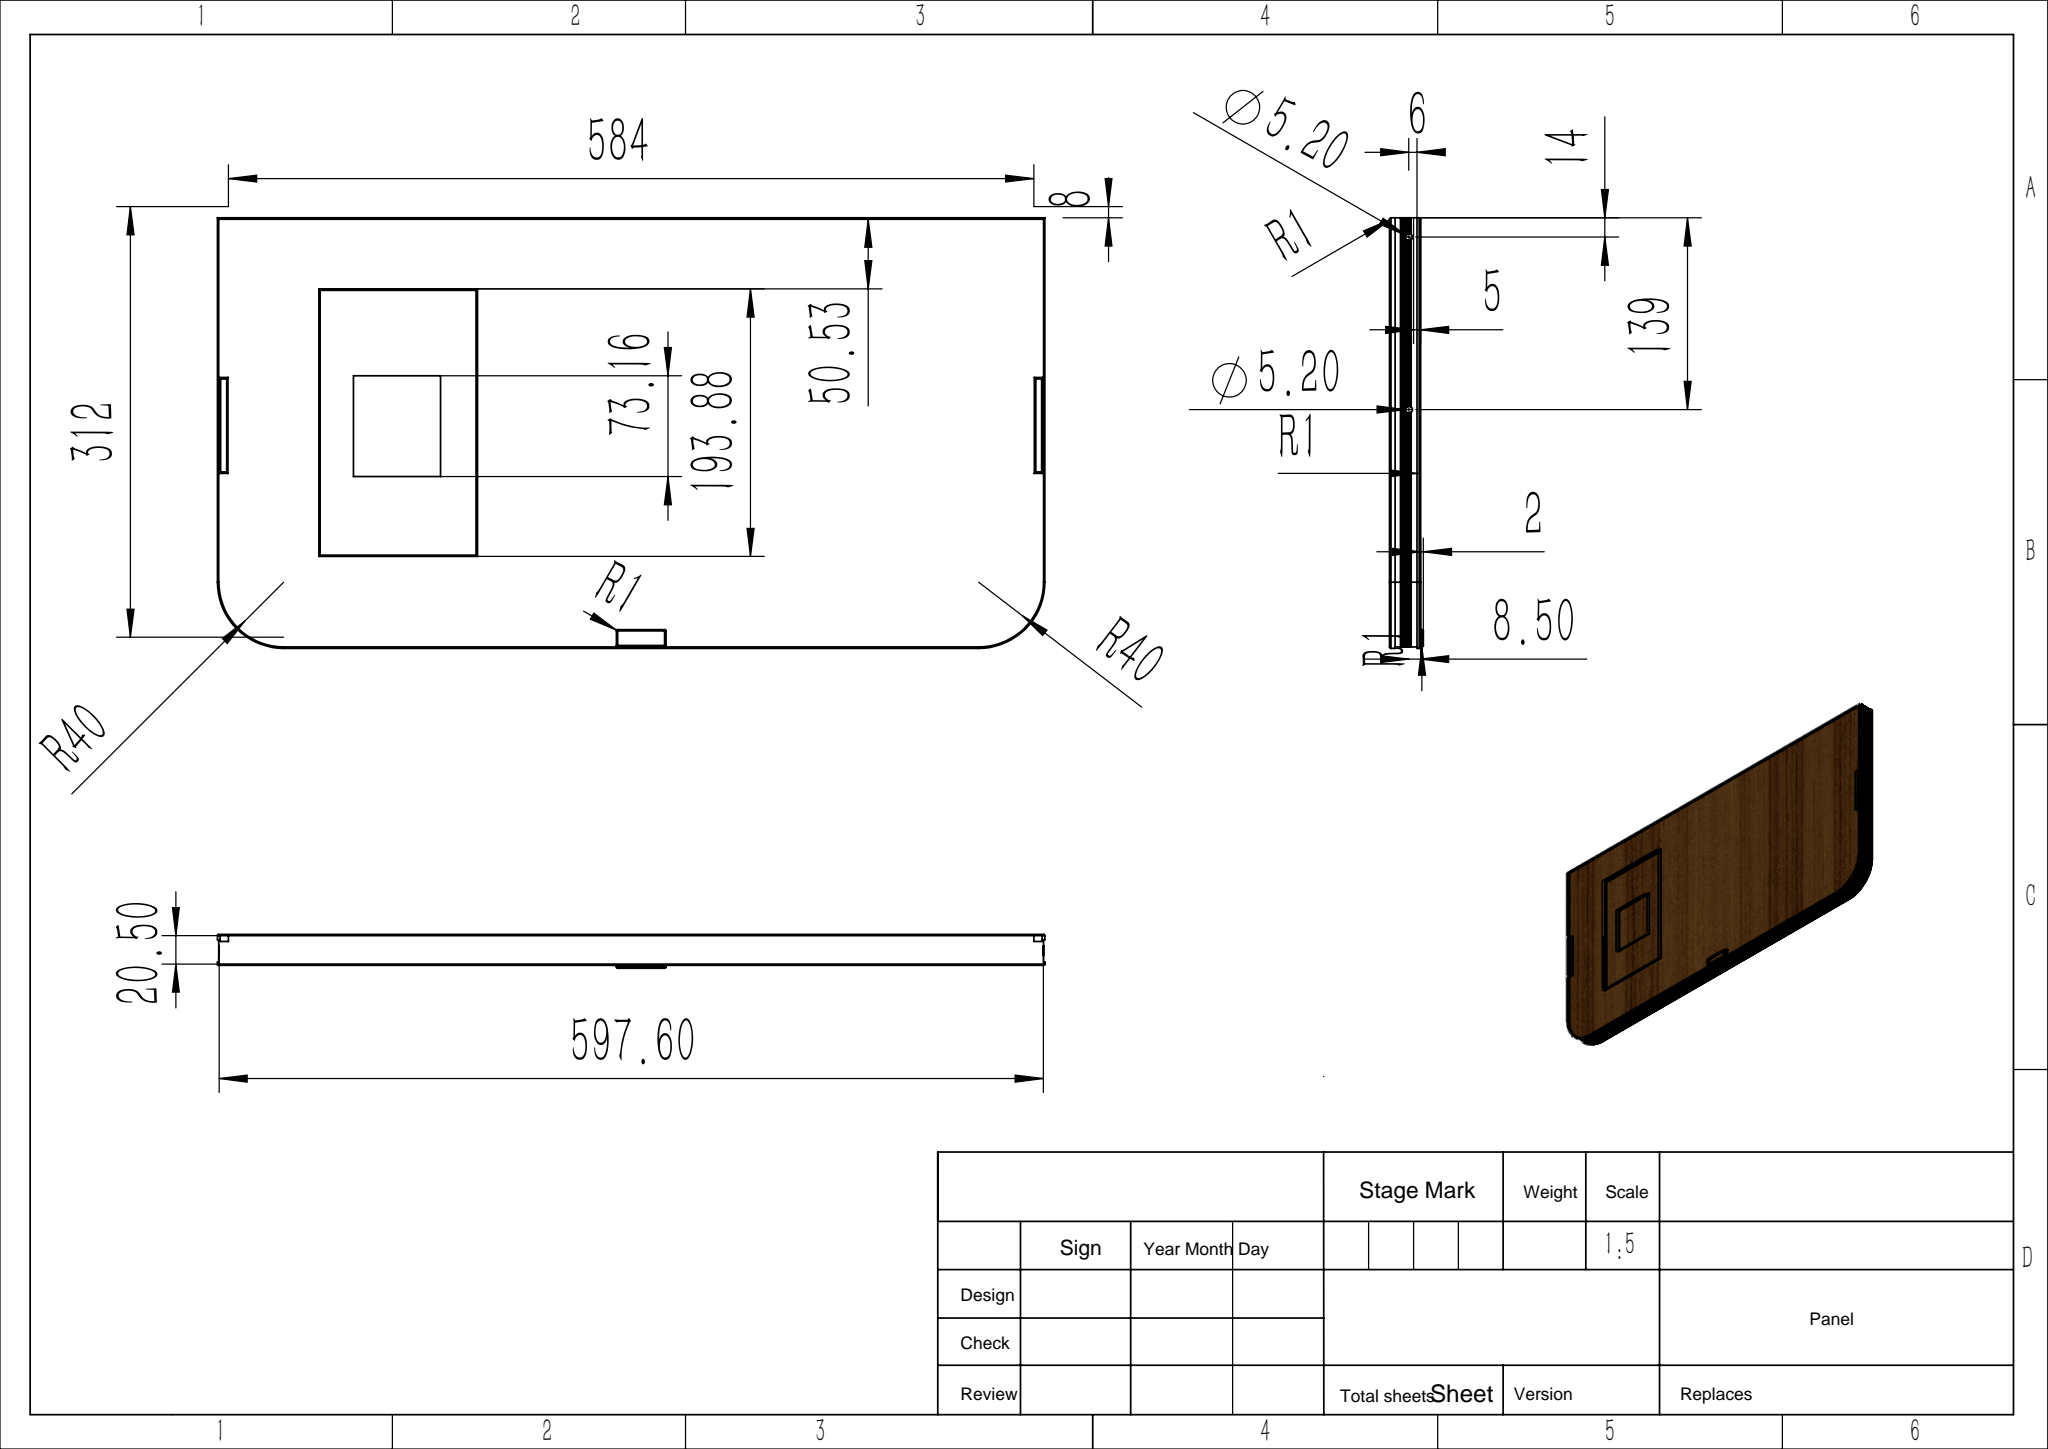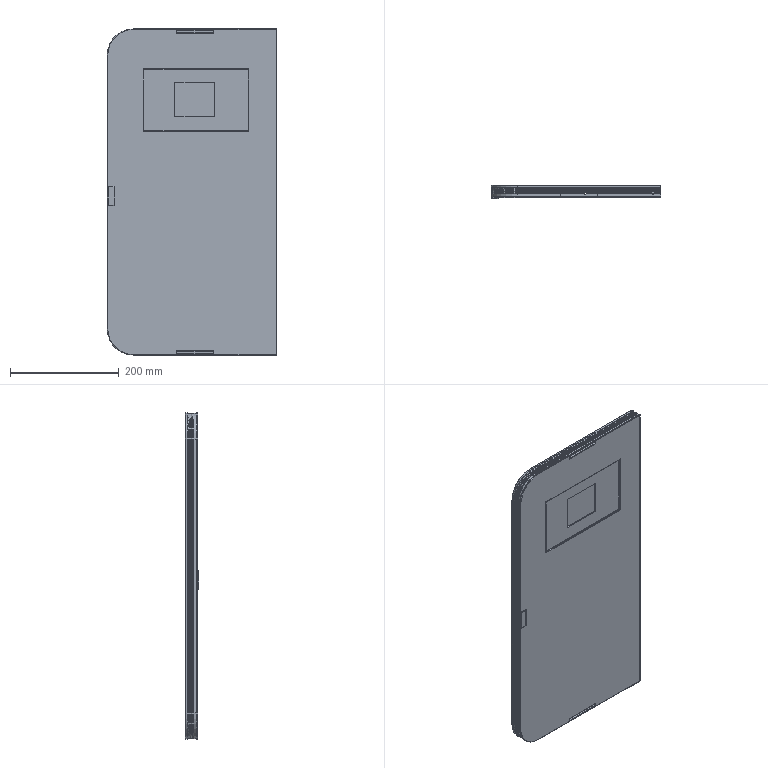Part | SolidWorks | features ICE 11, Fillet 4, MirrorPattern 1, Sweep 1 | 1 solid | 268 faces | box 312 x 24.5 x 600 mm | volume 4043732 mm3 | plane 166 | cylinder 50 | cone 44 | torus 4 | sphere 4 | commonest cylinder face diameters 2 x28 5.2 x10 94 x4 96 x4 80 x2 92 x2